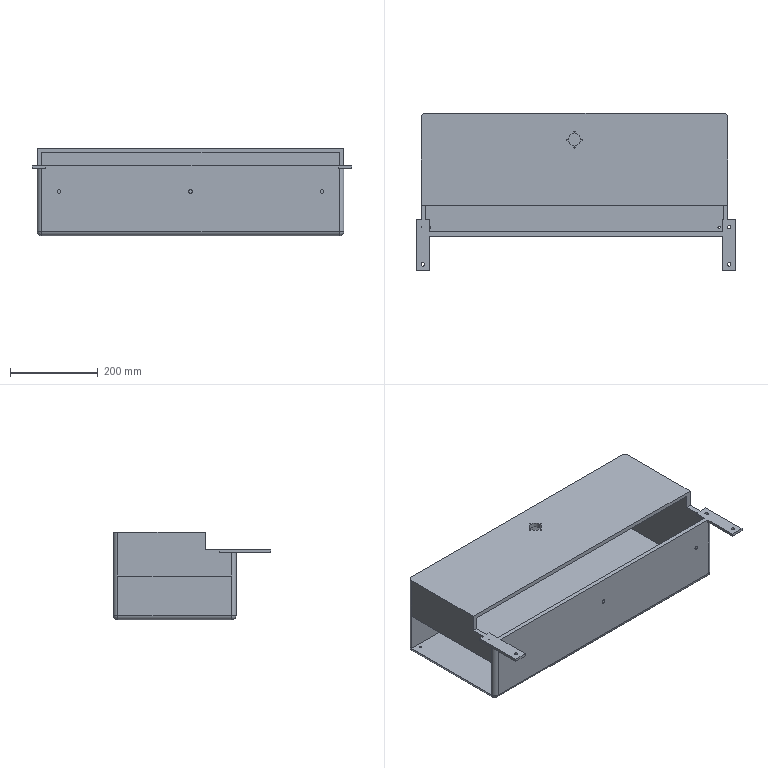Part | SolidWorks | features ICE 5, HoleWzd 3, Extrusion 1, Fillet 1, Shell 1 | 1 solid | 82 faces | box 730 x 359.087 x 200 mm | volume 6377520 mm3 | cylinder 39 | plane 31 | cone 8 | sphere 4 | commonest cylinder face diameters 2.5 x8 5 x8 20 x8 8.125 x7 8.5 x6 28 x2